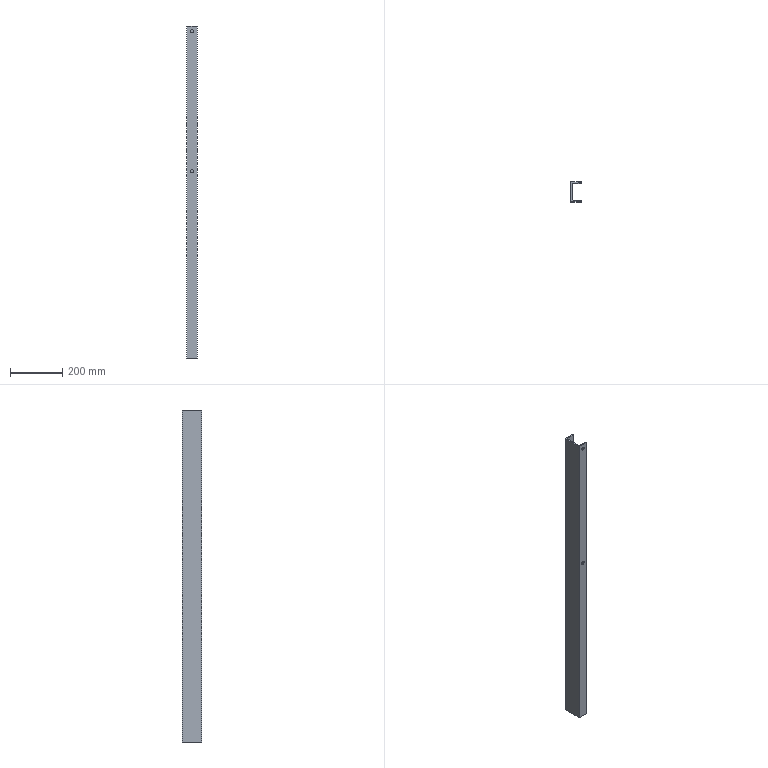Part | STEP file | BCC3 H13_6 | 1 solid | 14 faces | box 40 x 75 x 1270 mm | volume 877986 mm3 | plane 10 | cylinder 4 | commonest cylinder face diameters 12 x4
STEP:
#1=CARTESIAN_POINT('',(0.,0.,0.));
#2=DIRECTION('',(0.,0.,1.));
#3=DIRECTION('',(1.,0.,0.));
#4=AXIS2_PLACEMENT_3D('',#1,#2,#3);
#5=CARTESIAN_POINT('',(14.,-32.225,615.));
#6=VERTEX_POINT('',#5);
#7=CARTESIAN_POINT('',(14.,-37.5,615.));
#8=VERTEX_POINT('',#7);
#9=CARTESIAN_POINT('',(14.,-27.5,615.));
#10=DIRECTION('',(0.,-1.,0.));
#11=VECTOR('',#10,1.);
#12=LINE('',#9,#11);
#13=CARTESIAN_POINT('',(20.,-27.5,615.));
#14=DIRECTION('',(0.,-1.,0.));
#15=DIRECTION('',(-1.,0.,0.));
#16=AXIS2_PLACEMENT_3D('',#13,#14,#15);
#17=CYLINDRICAL_SURFACE('',#16,6.);
#18=CARTESIAN_POINT('',(6.283,0.));
#19=DIRECTION('',(0.,1.));
#20=VECTOR('',#19,1.);
#21=LINE('',#18,#20);
#22=(GEOMETRIC_REPRESENTATION_CONTEXT(2)PARAMETRIC_REPRESENTATION_CONTEXT()REPRESENTATION_CONTEXT('',''));
#23=DEFINITIONAL_REPRESENTATION('',(#21),#22);
#24=PCURVE('',#17,#23);
#25=CARTESIAN_POINT('',(20.,-27.5,615.));
#26=DIRECTION('',(0.,-1.,0.));
#27=DIRECTION('',(-1.,0.,0.));
#28=AXIS2_PLACEMENT_3D('',#25,#26,#27);
#29=CYLINDRICAL_SURFACE('',#28,6.);
#30=CARTESIAN_POINT('',(0.,0.));
#31=DIRECTION('',(0.,1.));
#32=VECTOR('',#31,1.);
#33=LINE('',#30,#32);
#34=(GEOMETRIC_REPRESENTATION_CONTEXT(2)PARAMETRIC_REPRESENTATION_CONTEXT()REPRESENTATION_CONTEXT('',''));
#35=DEFINITIONAL_REPRESENTATION('',(#33),#34);
#36=PCURVE('',#29,#35);
#37=SURFACE_CURVE('',#12,(#24,#36),.PCURVE_S1.);
#38=EDGE_CURVE('',#6,#8,#37,.T.);
#39=ORIENTED_EDGE('',*,*,#38,.T.);
#40=CARTESIAN_POINT('',(26.,-37.5,615.));
#41=VERTEX_POINT('',#40);
#42=CARTESIAN_POINT('',(20.,-37.5,615.));
#43=DIRECTION('',(0.,1.,0.));
#44=DIRECTION('',(1.,0.,0.));
#45=AXIS2_PLACEMENT_3D('',#42,#43,#44);
#46=CIRCLE('',#45,6.);
#47=CARTESIAN_POINT('',(9.425,10.));
#48=DIRECTION('',(-1.,0.));
#49=VECTOR('',#48,1.);
#50=LINE('',#47,#49);
#51=(GEOMETRIC_REPRESENTATION_CONTEXT(2)PARAMETRIC_REPRESENTATION_CONTEXT()REPRESENTATION_CONTEXT('',''));
#52=DEFINITIONAL_REPRESENTATION('',(#50),#51);
#53=PCURVE('',#17,#52);
#54=CARTESIAN_POINT('',(0.,-37.5,635.));
#55=DIRECTION('',(0.,1.,0.));
#56=DIRECTION('',(0.,0.,1.));
#57=AXIS2_PLACEMENT_3D('',#54,#55,#56);
#58=PLANE('',#57);
#59=CARTESIAN_POINT('',(-20.,20.));
#60=DIRECTION('',(0.,1.));
#61=AXIS2_PLACEMENT_2D('',#59,#60);
#62=CIRCLE('',#61,6.);
#63=(GEOMETRIC_REPRESENTATION_CONTEXT(2)PARAMETRIC_REPRESENTATION_CONTEXT()REPRESENTATION_CONTEXT('',''));
#64=DEFINITIONAL_REPRESENTATION('',(#62),#63);
#65=PCURVE('',#58,#64);
#66=SURFACE_CURVE('',#46,(#53,#65),.PCURVE_S1.);
#67=EDGE_CURVE('',#8,#41,#66,.T.);
#68=ORIENTED_EDGE('',*,*,#67,.T.);
#69=CARTESIAN_POINT('',(26.,-33.275,615.));
#70=VERTEX_POINT('',#69);
#71=CARTESIAN_POINT('',(26.,-27.5,615.));
#72=DIRECTION('',(0.,-1.,0.));
#73=VECTOR('',#72,1.);
#74=LINE('',#71,#73);
#75=CARTESIAN_POINT('',(3.142,0.));
#76=DIRECTION('',(0.,1.));
#77=VECTOR('',#76,1.);
#78=LINE('',#75,#77);
#79=(GEOMETRIC_REPRESENTATION_CONTEXT(2)PARAMETRIC_REPRESENTATION_CONTEXT()REPRESENTATION_CONTEXT('',''));
#80=DEFINITIONAL_REPRESENTATION('',(#78),#79);
#81=PCURVE('',#17,#80);
#82=CARTESIAN_POINT('',(3.142,0.));
#83=DIRECTION('',(0.,1.));
#84=VECTOR('',#83,1.);
#85=LINE('',#82,#84);
#86=(GEOMETRIC_REPRESENTATION_CONTEXT(2)PARAMETRIC_REPRESENTATION_CONTEXT()REPRESENTATION_CONTEXT('',''));
#87=DEFINITIONAL_REPRESENTATION('',(#85),#86);
#88=PCURVE('',#29,#87);
#89=SURFACE_CURVE('',#74,(#81,#88),.PCURVE_S1.);
#90=EDGE_CURVE('',#70,#41,#89,.T.);
#91=ORIENTED_EDGE('',*,*,#90,.F.);
#92=CARTESIAN_POINT('',(14.,-32.225,615.));
#93=CARTESIAN_POINT('',(14.,-32.225,627.));
#94=CARTESIAN_POINT('',(26.,-33.275,627.));
#95=CARTESIAN_POINT('',(26.,-33.275,615.));
#96=(BOUNDED_CURVE()B_SPLINE_CURVE(3,(#92,#93,#94,#95),.UNSPECIFIED.,.F.,.F.)B_SPLINE_CURVE_WITH_KNOTS((4,4),(3.142,6.283),.PIECEWISE_BEZIER_KNOTS.)CURVE()GEOMETRIC_REPRESENTATION_ITEM()RATIONAL_B_SPLINE_CURVE((1.,0.3333,0.3333,1.))REPRESENTATION_ITEM(''));
#97=CARTESIAN_POINT('',(6.283,4.725));
#98=CARTESIAN_POINT('',(6.253,4.725));
#99=CARTESIAN_POINT('',(6.19,4.727));
#100=CARTESIAN_POINT('',(6.085,4.735));
#101=CARTESIAN_POINT('',(5.972,4.749));
#102=CARTESIAN_POINT('',(5.848,4.773));
#103=CARTESIAN_POINT('',(5.713,4.807));
#104=CARTESIAN_POINT('',(5.567,4.853));
#105=CARTESIAN_POINT('',(5.412,4.911));
#106=CARTESIAN_POINT('',(5.246,4.982));
#107=CARTESIAN_POINT('',(5.073,5.064));
#108=CARTESIAN_POINT('',(4.894,5.155));
#109=CARTESIAN_POINT('',(4.712,5.25));
#110=CARTESIAN_POINT('',(4.531,5.346));
#111=CARTESIAN_POINT('',(4.352,5.436));
#112=CARTESIAN_POINT('',(4.179,5.519));
#113=CARTESIAN_POINT('',(4.013,5.59));
#114=CARTESIAN_POINT('',(3.857,5.648));
#115=CARTESIAN_POINT('',(3.712,5.694));
#116=CARTESIAN_POINT('',(3.577,5.727));
#117=CARTESIAN_POINT('',(3.453,5.751));
#118=CARTESIAN_POINT('',(3.339,5.766));
#119=CARTESIAN_POINT('',(3.235,5.774));
#120=CARTESIAN_POINT('',(3.172,5.775));
#121=CARTESIAN_POINT('',(3.142,5.775));
#122=B_SPLINE_CURVE_WITH_KNOTS('',3,(#97,#98,#99,#100,#101,#102,#103,#104,#105,#106,#107,#108,#109,#110,#111,#112,#113,#114,#115,#116,#117,#118,#119,#120,#121),.UNSPECIFIED.,.F.,.F.,(4,1,1,1,1,1,1,1,1,1,1,1,1,1,1,1,1,1,1,1,1,1,4),(3.142,3.284,3.427,3.57,3.713,3.856,3.998,4.141,4.284,4.427,4.57,4.712,4.855,4.998,5.141,5.284,5.426,5.569,5.712,5.855,5.998,6.14,6.283),.QUASI_UNIFORM_KNOTS.);
#123=(GEOMETRIC_REPRESENTATION_CONTEXT(2)PARAMETRIC_REPRESENTATION_CONTEXT()REPRESENTATION_CONTEXT('',''));
#124=DEFINITIONAL_REPRESENTATION('',(#122),#123);
#125=PCURVE('',#17,#124);
#126=CARTESIAN_POINT('',(40.,-34.5,635.));
#127=DIRECTION('',(-0.08716,-0.9962,0.));
#128=DIRECTION('',(0.9962,-0.08716,0.));
#129=AXIS2_PLACEMENT_3D('',#126,#127,#128);
#130=PLANE('',#129);
#131=CARTESIAN_POINT('',(-26.099,-20.));
#132=CARTESIAN_POINT('',(-26.099,-8.));
#133=CARTESIAN_POINT('',(-14.053,-8.));
#134=CARTESIAN_POINT('',(-14.053,-20.));
#135=(BOUNDED_CURVE()B_SPLINE_CURVE(3,(#131,#132,#133,#134),.UNSPECIFIED.,.F.,.F.)B_SPLINE_CURVE_WITH_KNOTS((4,4),(3.142,6.283),.PIECEWISE_BEZIER_KNOTS.)CURVE()GEOMETRIC_REPRESENTATION_ITEM()RATIONAL_B_SPLINE_CURVE((1.,0.3333,0.3333,1.))REPRESENTATION_ITEM(''));
#136=(GEOMETRIC_REPRESENTATION_CONTEXT(2)PARAMETRIC_REPRESENTATION_CONTEXT()REPRESENTATION_CONTEXT('',''));
#137=DEFINITIONAL_REPRESENTATION('',(#135),#136);
#138=PCURVE('',#130,#137);
#139=SURFACE_CURVE('',#96,(#125,#138),.PCURVE_S1.);
#140=EDGE_CURVE('',#6,#70,#139,.T.);
#141=ORIENTED_EDGE('',*,*,#140,.F.);
#142=EDGE_LOOP('',(#39,#68,#91,#141));
#143=FACE_BOUND('',#142,.F.);
#144=ADVANCED_FACE('',(#143),#17,.F.);
#145=CARTESIAN_POINT('',(14.,-32.225,80.));
#146=VERTEX_POINT('',#145);
#147=CARTESIAN_POINT('',(14.,-37.5,80.));
#148=VERTEX_POINT('',#147);
#149=CARTESIAN_POINT('',(14.,-27.5,80.));
#150=DIRECTION('',(0.,-1.,0.));
#151=VECTOR('',#150,1.);
#152=LINE('',#149,#151);
#153=CARTESIAN_POINT('',(20.,-27.5,80.));
#154=DIRECTION('',(0.,-1.,0.));
#155=DIRECTION('',(-1.,0.,0.));
#156=AXIS2_PLACEMENT_3D('',#153,#154,#155);
#157=CYLINDRICAL_SURFACE('',#156,6.);
#158=CARTESIAN_POINT('',(6.283,0.));
#159=DIRECTION('',(0.,1.));
#160=VECTOR('',#159,1.);
#161=LINE('',#158,#160);
#162=(GEOMETRIC_REPRESENTATION_CONTEXT(2)PARAMETRIC_REPRESENTATION_CONTEXT()REPRESENTATION_CONTEXT('',''));
#163=DEFINITIONAL_REPRESENTATION('',(#161),#162);
#164=PCURVE('',#157,#163);
#165=CARTESIAN_POINT('',(20.,-27.5,80.));
#166=DIRECTION('',(0.,-1.,0.));
#167=DIRECTION('',(-1.,0.,0.));
#168=AXIS2_PLACEMENT_3D('',#165,#166,#167);
#169=CYLINDRICAL_SURFACE('',#168,6.);
#170=CARTESIAN_POINT('',(0.,0.));
#171=DIRECTION('',(0.,1.));
#172=VECTOR('',#171,1.);
#173=LINE('',#170,#172);
#174=(GEOMETRIC_REPRESENTATION_CONTEXT(2)PARAMETRIC_REPRESENTATION_CONTEXT()REPRESENTATION_CONTEXT('',''));
#175=DEFINITIONAL_REPRESENTATION('',(#173),#174);
#176=PCURVE('',#169,#175);
#177=SURFACE_CURVE('',#152,(#164,#176),.PCURVE_S1.);
#178=EDGE_CURVE('',#146,#148,#177,.T.);
#179=ORIENTED_EDGE('',*,*,#178,.T.);
#180=CARTESIAN_POINT('',(26.,-37.5,80.));
#181=VERTEX_POINT('',#180);
#182=CARTESIAN_POINT('',(20.,-37.5,80.));
#183=DIRECTION('',(0.,1.,0.));
#184=DIRECTION('',(1.,0.,0.));
#185=AXIS2_PLACEMENT_3D('',#182,#183,#184);
#186=CIRCLE('',#185,6.);
#187=CARTESIAN_POINT('',(9.425,10.));
#188=DIRECTION('',(-1.,0.));
#189=VECTOR('',#188,1.);
#190=LINE('',#187,#189);
#191=(GEOMETRIC_REPRESENTATION_CONTEXT(2)PARAMETRIC_REPRESENTATION_CONTEXT()REPRESENTATION_CONTEXT('',''));
#192=DEFINITIONAL_REPRESENTATION('',(#190),#191);
#193=PCURVE('',#157,#192);
#194=CARTESIAN_POINT('',(-555.,20.));
#195=DIRECTION('',(0.,1.));
#196=AXIS2_PLACEMENT_2D('',#194,#195);
#197=CIRCLE('',#196,6.);
#198=(GEOMETRIC_REPRESENTATION_CONTEXT(2)PARAMETRIC_REPRESENTATION_CONTEXT()REPRESENTATION_CONTEXT('',''));
#199=DEFINITIONAL_REPRESENTATION('',(#197),#198);
#200=PCURVE('',#58,#199);
#201=SURFACE_CURVE('',#186,(#193,#200),.PCURVE_S1.);
#202=EDGE_CURVE('',#148,#181,#201,.T.);
#203=ORIENTED_EDGE('',*,*,#202,.T.);
#204=CARTESIAN_POINT('',(26.,-33.275,80.));
#205=VERTEX_POINT('',#204);
#206=CARTESIAN_POINT('',(26.,-27.5,80.));
#207=DIRECTION('',(0.,-1.,0.));
#208=VECTOR('',#207,1.);
#209=LINE('',#206,#208);
#210=CARTESIAN_POINT('',(3.142,0.));
#211=DIRECTION('',(0.,1.));
#212=VECTOR('',#211,1.);
#213=LINE('',#210,#212);
#214=(GEOMETRIC_REPRESENTATION_CONTEXT(2)PARAMETRIC_REPRESENTATION_CONTEXT()REPRESENTATION_CONTEXT('',''));
#215=DEFINITIONAL_REPRESENTATION('',(#213),#214);
#216=PCURVE('',#157,#215);
#217=CARTESIAN_POINT('',(3.142,0.));
#218=DIRECTION('',(0.,1.));
#219=VECTOR('',#218,1.);
#220=LINE('',#217,#219);
#221=(GEOMETRIC_REPRESENTATION_CONTEXT(2)PARAMETRIC_REPRESENTATION_CONTEXT()REPRESENTATION_CONTEXT('',''));
#222=DEFINITIONAL_REPRESENTATION('',(#220),#221);
#223=PCURVE('',#169,#222);
#224=SURFACE_CURVE('',#209,(#216,#223),.PCURVE_S1.);
#225=EDGE_CURVE('',#205,#181,#224,.T.);
#226=ORIENTED_EDGE('',*,*,#225,.F.);
#227=CARTESIAN_POINT('',(14.,-32.225,80.));
#228=CARTESIAN_POINT('',(14.,-32.225,92.));
#229=CARTESIAN_POINT('',(26.,-33.275,92.));
#230=CARTESIAN_POINT('',(26.,-33.275,80.));
#231=(BOUNDED_CURVE()B_SPLINE_CURVE(3,(#227,#228,#229,#230),.UNSPECIFIED.,.F.,.F.)B_SPLINE_CURVE_WITH_KNOTS((4,4),(3.142,6.283),.PIECEWISE_BEZIER_KNOTS.)CURVE()GEOMETRIC_REPRESENTATION_ITEM()RATIONAL_B_SPLINE_CURVE((1.,0.3333,0.3333,1.))REPRESENTATION_ITEM(''));
#232=CARTESIAN_POINT('',(6.283,4.725));
#233=CARTESIAN_POINT('',(6.253,4.725));
#234=CARTESIAN_POINT('',(6.19,4.727));
#235=CARTESIAN_POINT('',(6.085,4.735));
#236=CARTESIAN_POINT('',(5.972,4.749));
#237=CARTESIAN_POINT('',(5.848,4.773));
#238=CARTESIAN_POINT('',(5.713,4.807));
#239=CARTESIAN_POINT('',(5.567,4.853));
#240=CARTESIAN_POINT('',(5.412,4.911));
#241=CARTESIAN_POINT('',(5.246,4.982));
#242=CARTESIAN_POINT('',(5.073,5.064));
#243=CARTESIAN_POINT('',(4.894,5.155));
#244=CARTESIAN_POINT('',(4.712,5.25));
#245=CARTESIAN_POINT('',(4.531,5.346));
#246=CARTESIAN_POINT('',(4.352,5.436));
#247=CARTESIAN_POINT('',(4.179,5.519));
#248=CARTESIAN_POINT('',(4.013,5.59));
#249=CARTESIAN_POINT('',(3.857,5.648));
#250=CARTESIAN_POINT('',(3.712,5.694));
#251=CARTESIAN_POINT('',(3.577,5.727));
#252=CARTESIAN_POINT('',(3.453,5.751));
#253=CARTESIAN_POINT('',(3.339,5.766));
#254=CARTESIAN_POINT('',(3.235,5.774));
#255=CARTESIAN_POINT('',(3.172,5.775));
#256=CARTESIAN_POINT('',(3.142,5.775));
#257=B_SPLINE_CURVE_WITH_KNOTS('',3,(#232,#233,#234,#235,#236,#237,#238,#239,#240,#241,#242,#243,#244,#245,#246,#247,#248,#249,#250,#251,#252,#253,#254,#255,#256),.UNSPECIFIED.,.F.,.F.,(4,1,1,1,1,1,1,1,1,1,1,1,1,1,1,1,1,1,1,1,1,1,4),(3.142,3.284,3.427,3.57,3.713,3.856,3.998,4.141,4.284,4.427,4.57,4.712,4.855,4.998,5.141,5.284,5.426,5.569,5.712,5.855,5.998,6.14,6.283),.QUASI_UNIFORM_KNOTS.);
#258=(GEOMETRIC_REPRESENTATION_CONTEXT(2)PARAMETRIC_REPRESENTATION_CONTEXT()REPRESENTATION_CONTEXT('',''));
#259=DEFINITIONAL_REPRESENTATION('',(#257),#258);
#260=PCURVE('',#157,#259);
#261=CARTESIAN_POINT('',(-26.099,-555.));
#262=CARTESIAN_POINT('',(-26.099,-543.));
#263=CARTESIAN_POINT('',(-14.053,-543.));
#264=CARTESIAN_POINT('',(-14.053,-555.));
#265=(BOUNDED_CURVE()B_SPLINE_CURVE(3,(#261,#262,#263,#264),.UNSPECIFIED.,.F.,.F.)B_SPLINE_CURVE_WITH_KNOTS((4,4),(3.142,6.283),.PIECEWISE_BEZIER_KNOTS.)CURVE()GEOMETRIC_REPRESENTATION_ITEM()RATIONAL_B_SPLINE_CURVE((1.,0.3333,0.3333,1.))REPRESENTATION_ITEM(''));
#266=(GEOMETRIC_REPRESENTATION_CONTEXT(2)PARAMETRIC_REPRESENTATION_CONTEXT()REPRESENTATION_CONTEXT('',''));
#267=DEFINITIONAL_REPRESENTATION('',(#265),#266);
#268=PCURVE('',#130,#267);
#269=SURFACE_CURVE('',#231,(#260,#268),.PCURVE_S1.);
#270=EDGE_CURVE('',#146,#205,#269,.T.);
#271=ORIENTED_EDGE('',*,*,#270,.F.);
#272=EDGE_LOOP('',(#179,#203,#226,#271));
#273=FACE_BOUND('',#272,.F.);
#274=ADVANCED_FACE('',(#273),#157,.F.);
#275=ORIENTED_EDGE('',*,*,#202,.T.);
#276=CARTESIAN_POINT('',(20.,-37.5,80.));
#277=DIRECTION('',(0.,1.,0.));
#278=DIRECTION('',(1.,0.,0.));
#279=AXIS2_PLACEMENT_3D('',#276,#277,#278);
#280=CIRCLE('',#279,6.);
#281=CARTESIAN_POINT('',(-555.,20.));
#282=DIRECTION('',(0.,1.));
#283=AXIS2_PLACEMENT_2D('',#281,#282);
#284=CIRCLE('',#283,6.);
#285=(GEOMETRIC_REPRESENTATION_CONTEXT(2)PARAMETRIC_REPRESENTATION_CONTEXT()REPRESENTATION_CONTEXT('',''));
#286=DEFINITIONAL_REPRESENTATION('',(#284),#285);
#287=PCURVE('',#58,#286);
#288=CARTESIAN_POINT('',(3.142,10.));
#289=DIRECTION('',(-1.,0.));
#290=VECTOR('',#289,1.);
#291=LINE('',#288,#290);
#292=(GEOMETRIC_REPRESENTATION_CONTEXT(2)PARAMETRIC_REPRESENTATION_CONTEXT()REPRESENTATION_CONTEXT('',''));
#293=DEFINITIONAL_REPRESENTATION('',(#291),#292);
#294=PCURVE('',#169,#293);
#295=SURFACE_CURVE('',#280,(#287,#294),.PCURVE_S1.);
#296=EDGE_CURVE('',#181,#148,#295,.T.);
#297=ORIENTED_EDGE('',*,*,#296,.T.);
#298=EDGE_LOOP('',(#275,#297));
#299=FACE_BOUND('',#298,.T.);
#300=CARTESIAN_POINT('',(0.,-37.5,-635.));
#301=VERTEX_POINT('',#300);
#302=CARTESIAN_POINT('',(40.,-37.5,-635.));
#303=VERTEX_POINT('',#302);
#304=CARTESIAN_POINT('',(0.,-37.5,-635.));
#305=DIRECTION('',(1.,0.,0.));
#306=VECTOR('',#305,1.);
#307=LINE('',#304,#306);
#308=CARTESIAN_POINT('',(-1270.,0.));
#309=DIRECTION('',(0.,1.));
#310=VECTOR('',#309,1.);
#311=LINE('',#308,#310);
#312=(GEOMETRIC_REPRESENTATION_CONTEXT(2)PARAMETRIC_REPRESENTATION_CONTEXT()REPRESENTATION_CONTEXT('',''));
#313=DEFINITIONAL_REPRESENTATION('',(#311),#312);
#314=PCURVE('',#58,#313);
#315=CARTESIAN_POINT('',(0.,0.,-635.));
#316=DIRECTION('',(0.,0.,1.));
#317=DIRECTION('',(1.,0.,0.));
#318=AXIS2_PLACEMENT_3D('',#315,#316,#317);
#319=PLANE('',#318);
#320=CARTESIAN_POINT('',(0.,-37.5));
#321=DIRECTION('',(1.,0.));
#322=VECTOR('',#321,1.);
#323=LINE('',#320,#322);
#324=(GEOMETRIC_REPRESENTATION_CONTEXT(2)PARAMETRIC_REPRESENTATION_CONTEXT()REPRESENTATION_CONTEXT('',''));
#325=DEFINITIONAL_REPRESENTATION('',(#323),#324);
#326=PCURVE('',#319,#325);
#327=SURFACE_CURVE('',#307,(#314,#326),.PCURVE_S1.);
#328=EDGE_CURVE('',#301,#303,#327,.T.);
#329=ORIENTED_EDGE('',*,*,#328,.T.);
#330=CARTESIAN_POINT('',(40.,-37.5,635.));
#331=VERTEX_POINT('',#330);
#332=CARTESIAN_POINT('',(40.,-37.5,635.));
#333=DIRECTION('',(0.,0.,-1.));
#334=VECTOR('',#333,1.);
#335=LINE('',#332,#334);
#336=CARTESIAN_POINT('',(0.,40.));
#337=DIRECTION('',(-1.,0.));
#338=VECTOR('',#337,1.);
#339=LINE('',#336,#338);
#340=(GEOMETRIC_REPRESENTATION_CONTEXT(2)PARAMETRIC_REPRESENTATION_CONTEXT()REPRESENTATION_CONTEXT('',''));
#341=DEFINITIONAL_REPRESENTATION('',(#339),#340);
#342=PCURVE('',#58,#341);
#343=CARTESIAN_POINT('',(40.,-37.5,635.));
#344=DIRECTION('',(-1.,0.,0.));
#345=DIRECTION('',(0.,0.,1.));
#346=AXIS2_PLACEMENT_3D('',#343,#344,#345);
#347=PLANE('',#346);
#348=CARTESIAN_POINT('',(0.,0.));
#349=DIRECTION('',(-1.,0.));
#350=VECTOR('',#349,1.);
#351=LINE('',#348,#350);
#352=(GEOMETRIC_REPRESENTATION_CONTEXT(2)PARAMETRIC_REPRESENTATION_CONTEXT()REPRESENTATION_CONTEXT('',''));
#353=DEFINITIONAL_REPRESENTATION('',(#351),#352);
#354=PCURVE('',#347,#353);
#355=SURFACE_CURVE('',#335,(#342,#354),.PCURVE_S1.);
#356=EDGE_CURVE('',#331,#303,#355,.T.);
#357=ORIENTED_EDGE('',*,*,#356,.F.);
#358=CARTESIAN_POINT('',(0.,-37.5,635.));
#359=VERTEX_POINT('',#358);
#360=CARTESIAN_POINT('',(0.,-37.5,635.));
#361=DIRECTION('',(1.,0.,0.));
#362=VECTOR('',#361,1.);
#363=LINE('',#360,#362);
#364=CARTESIAN_POINT('',(0.,0.));
#365=DIRECTION('',(0.,1.));
#366=VECTOR('',#365,1.);
#367=LINE('',#364,#366);
#368=(GEOMETRIC_REPRESENTATION_CONTEXT(2)PARAMETRIC_REPRESENTATION_CONTEXT()REPRESENTATION_CONTEXT('',''));
#369=DEFINITIONAL_REPRESENTATION('',(#367),#368);
#370=PCURVE('',#58,#369);
#371=CARTESIAN_POINT('',(0.,0.,635.));
#372=DIRECTION('',(0.,0.,1.));
#373=DIRECTION('',(1.,0.,0.));
#374=AXIS2_PLACEMENT_3D('',#371,#372,#373);
#375=PLANE('',#374);
#376=CARTESIAN_POINT('',(0.,-37.5));
#377=DIRECTION('',(1.,0.));
#378=VECTOR('',#377,1.);
#379=LINE('',#376,#378);
#380=(GEOMETRIC_REPRESENTATION_CONTEXT(2)PARAMETRIC_REPRESENTATION_CONTEXT()REPRESENTATION_CONTEXT('',''));
#381=DEFINITIONAL_REPRESENTATION('',(#379),#380);
#382=PCURVE('',#375,#381);
#383=SURFACE_CURVE('',#363,(#370,#382),.PCURVE_S1.);
#384=EDGE_CURVE('',#359,#331,#383,.T.);
#385=ORIENTED_EDGE('',*,*,#384,.F.);
#386=CARTESIAN_POINT('',(0.,-37.5,635.));
#387=DIRECTION('',(0.,0.,-1.));
#388=VECTOR('',#387,1.);
#389=LINE('',#386,#388);
#390=CARTESIAN_POINT('',(0.,0.));
#391=DIRECTION('',(-1.,0.));
#392=VECTOR('',#391,1.);
#393=LINE('',#390,#392);
#394=(GEOMETRIC_REPRESENTATION_CONTEXT(2)PARAMETRIC_REPRESENTATION_CONTEXT()REPRESENTATION_CONTEXT('',''));
#395=DEFINITIONAL_REPRESENTATION('',(#393),#394);
#396=PCURVE('',#58,#395);
#397=CARTESIAN_POINT('',(0.,37.5,635.));
#398=DIRECTION('',(1.,0.,0.));
#399=DIRECTION('',(0.,0.,-1.));
#400=AXIS2_PLACEMENT_3D('',#397,#398,#399);
#401=PLANE('',#400);
#402=CARTESIAN_POINT('',(0.,-75.));
#403=DIRECTION('',(1.,0.));
#404=VECTOR('',#403,1.);
#405=LINE('',#402,#404);
#406=(GEOMETRIC_REPRESENTATION_CONTEXT(2)PARAMETRIC_REPRESENTATION_CONTEXT()REPRESENTATION_CONTEXT('',''));
#407=DEFINITIONAL_REPRESENTATION('',(#405),#406);
#408=PCURVE('',#401,#407);
#409=SURFACE_CURVE('',#389,(#396,#408),.PCURVE_S1.);
#410=EDGE_CURVE('',#359,#301,#409,.T.);
#411=ORIENTED_EDGE('',*,*,#410,.T.);
#412=EDGE_LOOP('',(#329,#357,#385,#411));
#413=FACE_BOUND('',#412,.T.);
#414=ORIENTED_EDGE('',*,*,#67,.T.);
#415=CARTESIAN_POINT('',(20.,-37.5,615.));
#416=DIRECTION('',(0.,1.,0.));
#417=DIRECTION('',(1.,0.,0.));
#418=AXIS2_PLACEMENT_3D('',#415,#416,#417);
#419=CIRCLE('',#418,6.);
#420=CARTESIAN_POINT('',(-20.,20.));
#421=DIRECTION('',(0.,1.));
#422=AXIS2_PLACEMENT_2D('',#420,#421);
#423=CIRCLE('',#422,6.);
#424=(GEOMETRIC_REPRESENTATION_CONTEXT(2)PARAMETRIC_REPRESENTATION_CONTEXT()REPRESENTATION_CONTEXT('',''));
#425=DEFINITIONAL_REPRESENTATION('',(#423),#424);
#426=PCURVE('',#58,#425);
#427=CARTESIAN_POINT('',(3.142,10.));
#428=DIRECTION('',(-1.,0.));
#429=VECTOR('',#428,1.);
#430=LINE('',#427,#429);
#431=(GEOMETRIC_REPRESENTATION_CONTEXT(2)PARAMETRIC_REPRESENTATION_CONTEXT()REPRESENTATION_CONTEXT('',''));
#432=DEFINITIONAL_REPRESENTATION('',(#430),#431);
#433=PCURVE('',#29,#432);
#434=SURFACE_CURVE('',#419,(#426,#433),.PCURVE_S1.);
#435=EDGE_CURVE('',#41,#8,#434,.T.);
#436=ORIENTED_EDGE('',*,*,#435,.T.);
#437=EDGE_LOOP('',(#414,#436));
#438=FACE_BOUND('',#437,.T.);
#439=ADVANCED_FACE('',(#299,#413,#438),#58,.F.);
#440=ORIENTED_EDGE('',*,*,#270,.F.);
#441=CARTESIAN_POINT('',(26.,-33.275,80.));
#442=CARTESIAN_POINT('',(26.,-33.275,68.));
#443=CARTESIAN_POINT('',(14.,-32.225,68.));
#444=CARTESIAN_POINT('',(14.,-32.225,80.));
#445=(BOUNDED_CURVE()B_SPLINE_CURVE(3,(#441,#442,#443,#444),.UNSPECIFIED.,.F.,.F.)B_SPLINE_CURVE_WITH_KNOTS((4,4),(0.,3.142),.PIECEWISE_BEZIER_KNOTS.)CURVE()GEOMETRIC_REPRESENTATION_ITEM()RATIONAL_B_SPLINE_CURVE((1.,0.3333,0.3333,1.))REPRESENTATION_ITEM(''));
#446=CARTESIAN_POINT('',(-14.053,-555.));
#447=CARTESIAN_POINT('',(-14.053,-567.));
#448=CARTESIAN_POINT('',(-26.099,-567.));
#449=CARTESIAN_POINT('',(-26.099,-555.));
#450=(BOUNDED_CURVE()B_SPLINE_CURVE(3,(#446,#447,#448,#449),.UNSPECIFIED.,.F.,.F.)B_SPLINE_CURVE_WITH_KNOTS((4,4),(0.,3.142),.PIECEWISE_BEZIER_KNOTS.)CURVE()GEOMETRIC_REPRESENTATION_ITEM()RATIONAL_B_SPLINE_CURVE((1.,0.3333,0.3333,1.))REPRESENTATION_ITEM(''));
#451=(GEOMETRIC_REPRESENTATION_CONTEXT(2)PARAMETRIC_REPRESENTATION_CONTEXT()REPRESENTATION_CONTEXT('',''));
#452=DEFINITIONAL_REPRESENTATION('',(#450),#451);
#453=PCURVE('',#130,#452);
#454=CARTESIAN_POINT('',(3.142,5.775));
#455=CARTESIAN_POINT('',(3.111,5.775));
#456=CARTESIAN_POINT('',(3.048,5.774));
#457=CARTESIAN_POINT('',(2.944,5.766));
#458=CARTESIAN_POINT('',(2.83,5.751));
#459=CARTESIAN_POINT('',(2.706,5.727));
#460=CARTESIAN_POINT('',(2.571,5.694));
#461=CARTESIAN_POINT('',(2.426,5.648));
#462=CARTESIAN_POINT('',(2.27,5.59));
#463=CARTESIAN_POINT('',(2.105,5.519));
#464=CARTESIAN_POINT('',(1.931,5.436));
#465=CARTESIAN_POINT('',(1.753,5.346));
#466=CARTESIAN_POINT('',(1.571,5.25));
#467=CARTESIAN_POINT('',(1.389,5.155));
#468=CARTESIAN_POINT('',(1.21,5.064));
#469=CARTESIAN_POINT('',(1.037,4.982));
#470=CARTESIAN_POINT('',(0.8717,4.911));
#471=CARTESIAN_POINT('',(0.7158,4.853));
#472=CARTESIAN_POINT('',(0.5703,4.807));
#473=CARTESIAN_POINT('',(0.4356,4.773));
#474=CARTESIAN_POINT('',(0.3115,4.749));
#475=CARTESIAN_POINT('',(0.1977,4.735));
#476=CARTESIAN_POINT('',(0.09367,4.727));
#477=CARTESIAN_POINT('',(0.0303,4.725));
#478=CARTESIAN_POINT('',(0.,4.725));
#479=B_SPLINE_CURVE_WITH_KNOTS('',3,(#454,#455,#456,#457,#458,#459,#460,#461,#462,#463,#464,#465,#466,#467,#468,#469,#470,#471,#472,#473,#474,#475,#476,#477,#478),.UNSPECIFIED.,.F.,.F.,(4,1,1,1,1,1,1,1,1,1,1,1,1,1,1,1,1,1,1,1,1,1,4),(0.,0.1428,0.2856,0.4284,0.5712,0.714,0.8568,0.9996,1.142,1.285,1.428,1.571,1.714,1.856,1.999,2.142,2.285,2.428,2.57,2.713,2.856,2.999,3.142),.QUASI_UNIFORM_KNOTS.);
#480=(GEOMETRIC_REPRESENTATION_CONTEXT(2)PARAMETRIC_REPRESENTATION_CONTEXT()REPRESENTATION_CONTEXT('',''));
#481=DEFINITIONAL_REPRESENTATION('',(#479),#480);
#482=PCURVE('',#169,#481);
#483=SURFACE_CURVE('',#445,(#453,#482),.PCURVE_S1.);
#484=EDGE_CURVE('',#205,#146,#483,.T.);
#485=ORIENTED_EDGE('',*,*,#484,.F.);
#486=EDGE_LOOP('',(#440,#485));
#487=FACE_BOUND('',#486,.T.);
#488=CARTESIAN_POINT('',(40.,-34.5,-635.));
#489=VERTEX_POINT('',#488);
#490=CARTESIAN_POINT('',(5.,-31.438,-635.));
#491=VERTEX_POINT('',#490);
#492=CARTESIAN_POINT('',(40.,-34.5,-635.));
#493=DIRECTION('',(-0.9962,0.08716,0.));
#494=VECTOR('',#493,1.);
#495=LINE('',#492,#494);
#496=CARTESIAN_POINT('',(0.,-1270.));
#497=DIRECTION('',(-1.,0.));
#498=VECTOR('',#497,1.);
#499=LINE('',#496,#498);
#500=(GEOMETRIC_REPRESENTATION_CONTEXT(2)PARAMETRIC_REPRESENTATION_CONTEXT()REPRESENTATION_CONTEXT('',''));
#501=DEFINITIONAL_REPRESENTATION('',(#499),#500);
#502=PCURVE('',#130,#501);
#503=CARTESIAN_POINT('',(40.,-34.5));
#504=DIRECTION('',(-0.9962,0.08716));
#505=VECTOR('',#504,1.);
#506=LINE('',#503,#505);
#507=(GEOMETRIC_REPRESENTATION_CONTEXT(2)PARAMETRIC_REPRESENTATION_CONTEXT()REPRESENTATION_CONTEXT('',''));
#508=DEFINITIONAL_REPRESENTATION('',(#506),#507);
#509=PCURVE('',#319,#508);
#510=SURFACE_CURVE('',#495,(#502,#509),.PCURVE_S1.);
#511=EDGE_CURVE('',#489,#491,#510,.T.);
#512=ORIENTED_EDGE('',*,*,#511,.T.);
#513=CARTESIAN_POINT('',(5.,-31.438,635.));
#514=VERTEX_POINT('',#513);
#515=CARTESIAN_POINT('',(5.,-31.438,635.));
#516=DIRECTION('',(0.,0.,-1.));
#517=VECTOR('',#516,1.);
#518=LINE('',#515,#517);
#519=CARTESIAN_POINT('',(-35.134,0.));
#520=DIRECTION('',(0.,-1.));
#521=VECTOR('',#520,1.);
#522=LINE('',#519,#521);
#523=(GEOMETRIC_REPRESENTATION_CONTEXT(2)PARAMETRIC_REPRESENTATION_CONTEXT()REPRESENTATION_CONTEXT('',''));
#524=DEFINITIONAL_REPRESENTATION('',(#522),#523);
#525=PCURVE('',#130,#524);
#526=CARTESIAN_POINT('',(5.,-31.438,635.));
#527=DIRECTION('',(-1.,0.,0.));
#528=DIRECTION('',(0.,0.,1.));
#529=AXIS2_PLACEMENT_3D('',#526,#527,#528);
#530=PLANE('',#529);
#531=CARTESIAN_POINT('',(0.,0.));
#532=DIRECTION('',(-1.,0.));
#533=VECTOR('',#532,1.);
#534=LINE('',#531,#533);
#535=(GEOMETRIC_REPRESENTATION_CONTEXT(2)PARAMETRIC_REPRESENTATION_CONTEXT()REPRESENTATION_CONTEXT('',''));
#536=DEFINITIONAL_REPRESENTATION('',(#534),#535);
#537=PCURVE('',#530,#536);
#538=SURFACE_CURVE('',#518,(#525,#537),.PCURVE_S1.);
#539=EDGE_CURVE('',#514,#491,#538,.T.);
#540=ORIENTED_EDGE('',*,*,#539,.F.);
#541=CARTESIAN_POINT('',(40.,-34.5,635.));
#542=VERTEX_POINT('',#541);
#543=CARTESIAN_POINT('',(40.,-34.5,635.));
#544=DIRECTION('',(-0.9962,0.08716,0.));
#545=VECTOR('',#544,1.);
#546=LINE('',#543,#545);
#547=CARTESIAN_POINT('',(0.,0.));
#548=DIRECTION('',(-1.,0.));
#549=VECTOR('',#548,1.);
#550=LINE('',#547,#549);
#551=(GEOMETRIC_REPRESENTATION_CONTEXT(2)PARAMETRIC_REPRESENTATION_CONTEXT()REPRESENTATION_CONTEXT('',''));
#552=DEFINITIONAL_REPRESENTATION('',(#550),#551);
#553=PCURVE('',#130,#552);
#554=CARTESIAN_POINT('',(40.,-34.5));
#555=DIRECTION('',(-0.9962,0.08716));
#556=VECTOR('',#555,1.);
#557=LINE('',#554,#556);
#558=(GEOMETRIC_REPRESENTATION_CONTEXT(2)PARAMETRIC_REPRESENTATION_CONTEXT()REPRESENTATION_CONTEXT('',''));
#559=DEFINITIONAL_REPRESENTATION('',(#557),#558);
#560=PCURVE('',#375,#559);
#561=SURFACE_CURVE('',#546,(#553,#560),.PCURVE_S1.);
#562=EDGE_CURVE('',#542,#514,#561,.T.);
#563=ORIENTED_EDGE('',*,*,#562,.F.);
#564=CARTESIAN_POINT('',(40.,-34.5,635.));
#565=DIRECTION('',(0.,0.,-1.));
#566=VECTOR('',#565,1.);
#567=LINE('',#564,#566);
#568=CARTESIAN_POINT('',(0.,0.));
#569=DIRECTION('',(0.,-1.));
#570=VECTOR('',#569,1.);
#571=LINE('',#568,#570);
#572=(GEOMETRIC_REPRESENTATION_CONTEXT(2)PARAMETRIC_REPRESENTATION_CONTEXT()REPRESENTATION_CONTEXT('',''));
#573=DEFINITIONAL_REPRESENTATION('',(#571),#572);
#574=PCURVE('',#130,#573);
#575=CARTESIAN_POINT('',(0.,3.));
#576=DIRECTION('',(-1.,0.));
#577=VECTOR('',#576,1.);
#578=LINE('',#575,#577);
#579=(GEOMETRIC_REPRESENTATION_CONTEXT(2)PARAMETRIC_REPRESENTATION_CONTEXT()REPRESENTATION_CONTEXT('',''));
#580=DEFINITIONAL_REPRESENTATION('',(#578),#579);
#581=PCURVE('',#347,#580);
#582=SURFACE_CURVE('',#567,(#574,#581),.PCURVE_S1.);
#583=EDGE_CURVE('',#542,#489,#582,.T.);
#584=ORIENTED_EDGE('',*,*,#583,.T.);
#585=EDGE_LOOP('',(#512,#540,#563,#584));
#586=FACE_BOUND('',#585,.T.);
#587=ORIENTED_EDGE('',*,*,#140,.F.);
#588=CARTESIAN_POINT('',(26.,-33.275,615.));
#589=CARTESIAN_POINT('',(26.,-33.275,603.));
#590=CARTESIAN_POINT('',(14.,-32.225,603.));
#591=CARTESIAN_POINT('',(14.,-32.225,615.));
#592=(BOUNDED_CURVE()B_SPLINE_CURVE(3,(#588,#589,#590,#591),.UNSPECIFIED.,.F.,.F.)B_SPLINE_CURVE_WITH_KNOTS((4,4),(0.,3.142),.PIECEWISE_BEZIER_KNOTS.)CURVE()GEOMETRIC_REPRESENTATION_ITEM()RATIONAL_B_SPLINE_CURVE((1.,0.3333,0.3333,1.))REPRESENTATION_ITEM(''));
#593=CARTESIAN_POINT('',(-14.053,-20.));
#594=CARTESIAN_POINT('',(-14.053,-32.));
#595=CARTESIAN_POINT('',(-26.099,-32.));
#596=CARTESIAN_POINT('',(-26.099,-20.));
#597=(BOUNDED_CURVE()B_SPLINE_CURVE(3,(#593,#594,#595,#596),.UNSPECIFIED.,.F.,.F.)B_SPLINE_CURVE_WITH_KNOTS((4,4),(0.,3.142),.PIECEWISE_BEZIER_KNOTS.)CURVE()GEOMETRIC_REPRESENTATION_ITEM()RATIONAL_B_SPLINE_CURVE((1.,0.3333,0.3333,1.))REPRESENTATION_ITEM(''));
#598=(GEOMETRIC_REPRESENTATION_CONTEXT(2)PARAMETRIC_REPRESENTATION_CONTEXT()REPRESENTATION_CONTEXT('',''));
#599=DEFINITIONAL_REPRESENTATION('',(#597),#598);
#600=PCURVE('',#130,#599);
#601=CARTESIAN_POINT('',(3.142,5.775));
#602=CARTESIAN_POINT('',(3.111,5.775));
#603=CARTESIAN_POINT('',(3.048,5.774));
#604=CARTESIAN_POINT('',(2.944,5.766));
#605=CARTESIAN_POINT('',(2.83,5.751));
#606=CARTESIAN_POINT('',(2.706,5.727));
#607=CARTESIAN_POINT('',(2.571,5.694));
#608=CARTESIAN_POINT('',(2.426,5.648));
#609=CARTESIAN_POINT('',(2.27,5.59));
#610=CARTESIAN_POINT('',(2.105,5.519));
#611=CARTESIAN_POINT('',(1.931,5.436));
#612=CARTESIAN_POINT('',(1.753,5.346));
#613=CARTESIAN_POINT('',(1.571,5.25));
#614=CARTESIAN_POINT('',(1.389,5.155));
#615=CARTESIAN_POINT('',(1.21,5.064));
#616=CARTESIAN_POINT('',(1.037,4.982));
#617=CARTESIAN_POINT('',(0.8717,4.911));
#618=CARTESIAN_POINT('',(0.7158,4.853));
#619=CARTESIAN_POINT('',(0.5703,4.807));
#620=CARTESIAN_POINT('',(0.4356,4.773));
#621=CARTESIAN_POINT('',(0.3115,4.749));
#622=CARTESIAN_POINT('',(0.1977,4.735));
#623=CARTESIAN_POINT('',(0.09367,4.727));
#624=CARTESIAN_POINT('',(0.0303,4.725));
#625=CARTESIAN_POINT('',(0.,4.725));
#626=B_SPLINE_CURVE_WITH_KNOTS('',3,(#601,#602,#603,#604,#605,#606,#607,#608,#609,#610,#611,#612,#613,#614,#615,#616,#617,#618,#619,#620,#621,#622,#623,#624,#625),.UNSPECIFIED.,.F.,.F.,(4,1,1,1,1,1,1,1,1,1,1,1,1,1,1,1,1,1,1,1,1,1,4),(0.,0.1428,0.2856,0.4284,0.5712,0.714,0.8568,0.9996,1.142,1.285,1.428,1.571,1.714,1.856,1.999,2.142,2.285,2.428,2.57,2.713,2.856,2.999,3.142),.QUASI_UNIFORM_KNOTS.);
#627=(GEOMETRIC_REPRESENTATION_CONTEXT(2)PARAMETRIC_REPRESENTATION_CONTEXT()REPRESENTATION_CONTEXT('',''));
#628=DEFINITIONAL_REPRESENTATION('',(#626),#627);
#629=PCURVE('',#29,#628);
#630=SURFACE_CURVE('',#592,(#600,#629),.PCURVE_S1.);
#631=EDGE_CURVE('',#70,#6,#630,.T.);
#632=ORIENTED_EDGE('',*,*,#631,.F.);
#633=EDGE_LOOP('',(#587,#632));
#634=FACE_BOUND('',#633,.T.);
#635=ADVANCED_FACE('',(#487,#586,#634),#130,.F.);
#636=CARTESIAN_POINT('',(40.,37.5,-635.));
#637=VERTEX_POINT('',#636);
#638=CARTESIAN_POINT('',(0.,37.5,-635.));
#639=VERTEX_POINT('',#638);
#640=CARTESIAN_POINT('',(40.,37.5,-635.));
#641=DIRECTION('',(-1.,0.,0.));
#642=VECTOR('',#641,1.);
#643=LINE('',#640,#642);
#644=CARTESIAN_POINT('',(40.,37.5,635.));
#645=DIRECTION('',(0.,-1.,0.));
#646=DIRECTION('',(0.,0.,-1.));
#647=AXIS2_PLACEMENT_3D('',#644,#645,#646);
#648=PLANE('',#647);
#649=CARTESIAN_POINT('',(1270.,0.));
#650=DIRECTION('',(0.,-1.));
#651=VECTOR('',#650,1.);
#652=LINE('',#649,#651);
#653=(GEOMETRIC_REPRESENTATION_CONTEXT(2)PARAMETRIC_REPRESENTATION_CONTEXT()REPRESENTATION_CONTEXT('',''));
#654=DEFINITIONAL_REPRESENTATION('',(#652),#653);
#655=PCURVE('',#648,#654);
#656=CARTESIAN_POINT('',(40.,37.5));
#657=DIRECTION('',(-1.,0.));
#658=VECTOR('',#657,1.);
#659=LINE('',#656,#658);
#660=(GEOMETRIC_REPRESENTATION_CONTEXT(2)PARAMETRIC_REPRESENTATION_CONTEXT()REPRESENTATION_CONTEXT('',''));
#661=DEFINITIONAL_REPRESENTATION('',(#659),#660);
#662=PCURVE('',#319,#661);
#663=SURFACE_CURVE('',#643,(#655,#662),.PCURVE_S1.);
#664=EDGE_CURVE('',#637,#639,#663,.T.);
#665=ORIENTED_EDGE('',*,*,#664,.T.);
#666=CARTESIAN_POINT('',(0.,37.5,635.));
#667=VERTEX_POINT('',#666);
#668=CARTESIAN_POINT('',(0.,37.5,635.));
#669=DIRECTION('',(0.,0.,-1.));
#670=VECTOR('',#669,1.);
#671=LINE('',#668,#670);
#672=CARTESIAN_POINT('',(0.,-40.));
#673=DIRECTION('',(1.,0.));
#674=VECTOR('',#673,1.);
#675=LINE('',#672,#674);
#676=(GEOMETRIC_REPRESENTATION_CONTEXT(2)PARAMETRIC_REPRESENTATION_CONTEXT()REPRESENTATION_CONTEXT('',''));
#677=DEFINITIONAL_REPRESENTATION('',(#675),#676);
#678=PCURVE('',#648,#677);
#679=CARTESIAN_POINT('',(0.,0.));
#680=DIRECTION('',(1.,0.));
#681=VECTOR('',#680,1.);
#682=LINE('',#679,#681);
#683=(GEOMETRIC_REPRESENTATION_CONTEXT(2)PARAMETRIC_REPRESENTATION_CONTEXT()REPRESENTATION_CONTEXT('',''));
#684=DEFINITIONAL_REPRESENTATION('',(#682),#683);
#685=PCURVE('',#401,#684);
#686=SURFACE_CURVE('',#671,(#678,#685),.PCURVE_S1.);
#687=EDGE_CURVE('',#667,#639,#686,.T.);
#688=ORIENTED_EDGE('',*,*,#687,.F.);
#689=CARTESIAN_POINT('',(40.,37.5,635.));
#690=VERTEX_POINT('',#689);
#691=CARTESIAN_POINT('',(40.,37.5,635.));
#692=DIRECTION('',(-1.,0.,0.));
#693=VECTOR('',#692,1.);
#694=LINE('',#691,#693);
#695=CARTESIAN_POINT('',(0.,0.));
#696=DIRECTION('',(0.,-1.));
#697=VECTOR('',#696,1.);
#698=LINE('',#695,#697);
#699=(GEOMETRIC_REPRESENTATION_CONTEXT(2)PARAMETRIC_REPRESENTATION_CONTEXT()REPRESENTATION_CONTEXT('',''));
#700=DEFINITIONAL_REPRESENTATION('',(#698),#699);
#701=PCURVE('',#648,#700);
#702=CARTESIAN_POINT('',(40.,37.5));
#703=DIRECTION('',(-1.,0.));
#704=VECTOR('',#703,1.);
#705=LINE('',#702,#704);
#706=(GEOMETRIC_REPRESENTATION_CONTEXT(2)PARAMETRIC_REPRESENTATION_CONTEXT()REPRESENTATION_CONTEXT('',''));
#707=DEFINITIONAL_REPRESENTATION('',(#705),#706);
#708=PCURVE('',#375,#707);
#709=SURFACE_CURVE('',#694,(#701,#708),.PCURVE_S1.);
#710=EDGE_CURVE('',#690,#667,#709,.T.);
#711=ORIENTED_EDGE('',*,*,#710,.F.);
#712=CARTESIAN_POINT('',(40.,37.5,635.));
#713=DIRECTION('',(0.,0.,-1.));
#714=VECTOR('',#713,1.);
#715=LINE('',#712,#714);
#716=CARTESIAN_POINT('',(0.,0.));
#717=DIRECTION('',(1.,0.));
#718=VECTOR('',#717,1.);
#719=LINE('',#716,#718);
#720=(GEOMETRIC_REPRESENTATION_CONTEXT(2)PARAMETRIC_REPRESENTATION_CONTEXT()REPRESENTATION_CONTEXT('',''));
#721=DEFINITIONAL_REPRESENTATION('',(#719),#720);
#722=PCURVE('',#648,#721);
#723=CARTESIAN_POINT('',(40.,34.5,635.));
#724=DIRECTION('',(-1.,0.,0.));
#725=DIRECTION('',(0.,0.,1.));
#726=AXIS2_PLACEMENT_3D('',#723,#724,#725);
#727=PLANE('',#726);
#728=CARTESIAN_POINT('',(0.,3.));
#729=DIRECTION('',(-1.,0.));
#730=VECTOR('',#729,1.);
#731=LINE('',#728,#730);
#732=(GEOMETRIC_REPRESENTATION_CONTEXT(2)PARAMETRIC_REPRESENTATION_CONTEXT()REPRESENTATION_CONTEXT('',''));
#733=DEFINITIONAL_REPRESENTATION('',(#731),#732);
#734=PCURVE('',#727,#733);
#735=SURFACE_CURVE('',#715,(#722,#734),.PCURVE_S1.);
#736=EDGE_CURVE('',#690,#637,#735,.T.);
#737=ORIENTED_EDGE('',*,*,#736,.T.);
#738=EDGE_LOOP('',(#665,#688,#711,#737));
#739=FACE_BOUND('',#738,.T.);
#740=ADVANCED_FACE('',(#739),#648,.F.);
#741=CARTESIAN_POINT('',(0.,37.5,-635.));
#742=DIRECTION('',(0.,-1.,0.));
#743=VECTOR('',#742,1.);
#744=LINE('',#741,#743);
#745=CARTESIAN_POINT('',(1270.,0.));
#746=DIRECTION('',(0.,-1.));
#747=VECTOR('',#746,1.);
#748=LINE('',#745,#747);
#749=(GEOMETRIC_REPRESENTATION_CONTEXT(2)PARAMETRIC_REPRESENTATION_CONTEXT()REPRESENTATION_CONTEXT('',''));
#750=DEFINITIONAL_REPRESENTATION('',(#748),#749);
#751=PCURVE('',#401,#750);
#752=CARTESIAN_POINT('',(0.,37.5));
#753=DIRECTION('',(0.,-1.));
#754=VECTOR('',#753,1.);
#755=LINE('',#752,#754);
#756=(GEOMETRIC_REPRESENTATION_CONTEXT(2)PARAMETRIC_REPRESENTATION_CONTEXT()REPRESENTATION_CONTEXT('',''));
#757=DEFINITIONAL_REPRESENTATION('',(#755),#756);
#758=PCURVE('',#319,#757);
#759=SURFACE_CURVE('',#744,(#751,#758),.PCURVE_S1.);
#760=EDGE_CURVE('',#639,#301,#759,.T.);
#761=ORIENTED_EDGE('',*,*,#760,.T.);
#762=ORIENTED_EDGE('',*,*,#410,.F.);
#763=CARTESIAN_POINT('',(0.,37.5,635.));
#764=DIRECTION('',(0.,-1.,0.));
#765=VECTOR('',#764,1.);
#766=LINE('',#763,#765);
#767=CARTESIAN_POINT('',(0.,0.));
#768=DIRECTION('',(0.,-1.));
#769=VECTOR('',#768,1.);
#770=LINE('',#767,#769);
#771=(GEOMETRIC_REPRESENTATION_CONTEXT(2)PARAMETRIC_REPRESENTATION_CONTEXT()REPRESENTATION_CONTEXT('',''));
#772=DEFINITIONAL_REPRESENTATION('',(#770),#771);
#773=PCURVE('',#401,#772);
#774=CARTESIAN_POINT('',(0.,37.5));
#775=DIRECTION('',(0.,-1.));
#776=VECTOR('',#775,1.);
#777=LINE('',#774,#776);
#778=(GEOMETRIC_REPRESENTATION_CONTEXT(2)PARAMETRIC_REPRESENTATION_CONTEXT()REPRESENTATION_CONTEXT('',''));
#779=DEFINITIONAL_REPRESENTATION('',(#777),#778);
#780=PCURVE('',#375,#779);
#781=SURFACE_CURVE('',#766,(#773,#780),.PCURVE_S1.);
#782=EDGE_CURVE('',#667,#359,#781,.T.);
#783=ORIENTED_EDGE('',*,*,#782,.F.);
#784=ORIENTED_EDGE('',*,*,#687,.T.);
#785=EDGE_LOOP('',(#761,#762,#783,#784));
#786=FACE_BOUND('',#785,.T.);
#787=ADVANCED_FACE('',(#786),#401,.F.);
#788=CARTESIAN_POINT('',(40.,-37.5,-635.));
#789=DIRECTION('',(0.,1.,0.));
#790=VECTOR('',#789,1.);
#791=LINE('',#788,#790);
#792=CARTESIAN_POINT('',(-1270.,0.));
#793=DIRECTION('',(0.,1.));
#794=VECTOR('',#793,1.);
#795=LINE('',#792,#794);
#796=(GEOMETRIC_REPRESENTATION_CONTEXT(2)PARAMETRIC_REPRESENTATION_CONTEXT()REPRESENTATION_CONTEXT('',''));
#797=DEFINITIONAL_REPRESENTATION('',(#795),#796);
#798=PCURVE('',#347,#797);
#799=CARTESIAN_POINT('',(40.,-37.5));
#800=DIRECTION('',(0.,1.));
#801=VECTOR('',#800,1.);
#802=LINE('',#799,#801);
#803=(GEOMETRIC_REPRESENTATION_CONTEXT(2)PARAMETRIC_REPRESENTATION_CONTEXT()REPRESENTATION_CONTEXT('',''));
#804=DEFINITIONAL_REPRESENTATION('',(#802),#803);
#805=PCURVE('',#319,#804);
#806=SURFACE_CURVE('',#791,(#798,#805),.PCURVE_S1.);
#807=EDGE_CURVE('',#303,#489,#806,.T.);
#808=ORIENTED_EDGE('',*,*,#807,.T.);
#809=ORIENTED_EDGE('',*,*,#583,.F.);
#810=CARTESIAN_POINT('',(40.,-37.5,635.));
#811=DIRECTION('',(0.,1.,0.));
#812=VECTOR('',#811,1.);
#813=LINE('',#810,#812);
#814=CARTESIAN_POINT('',(0.,0.));
#815=DIRECTION('',(0.,1.));
#816=VECTOR('',#815,1.);
#817=LINE('',#814,#816);
#818=(GEOMETRIC_REPRESENTATION_CONTEXT(2)PARAMETRIC_REPRESENTATION_CONTEXT()REPRESENTATION_CONTEXT('',''));
#819=DEFINITIONAL_REPRESENTATION('',(#817),#818);
#820=PCURVE('',#347,#819);
#821=CARTESIAN_POINT('',(40.,-37.5));
#822=DIRECTION('',(0.,1.));
#823=VECTOR('',#822,1.);
#824=LINE('',#821,#823);
#825=(GEOMETRIC_REPRESENTATION_CONTEXT(2)PARAMETRIC_REPRESENTATION_CONTEXT()REPRESENTATION_CONTEXT('',''));
#826=DEFINITIONAL_REPRESENTATION('',(#824),#825);
#827=PCURVE('',#375,#826);
#828=SURFACE_CURVE('',#813,(#820,#827),.PCURVE_S1.);
#829=EDGE_CURVE('',#331,#542,#828,.T.);
#830=ORIENTED_EDGE('',*,*,#829,.F.);
#831=ORIENTED_EDGE('',*,*,#356,.T.);
#832=EDGE_LOOP('',(#808,#809,#830,#831));
#833=FACE_BOUND('',#832,.T.);
#834=ADVANCED_FACE('',(#833),#347,.F.);
#835=CARTESIAN_POINT('',(5.,31.438,-635.));
#836=VERTEX_POINT('',#835);
#837=CARTESIAN_POINT('',(5.,-31.438,-635.));
#838=DIRECTION('',(0.,1.,0.));
#839=VECTOR('',#838,1.);
#840=LINE('',#837,#839);
#841=CARTESIAN_POINT('',(-1270.,0.));
#842=DIRECTION('',(0.,1.));
#843=VECTOR('',#842,1.);
#844=LINE('',#841,#843);
#845=(GEOMETRIC_REPRESENTATION_CONTEXT(2)PARAMETRIC_REPRESENTATION_CONTEXT()REPRESENTATION_CONTEXT('',''));
#846=DEFINITIONAL_REPRESENTATION('',(#844),#845);
#847=PCURVE('',#530,#846);
#848=CARTESIAN_POINT('',(5.,-31.438));
#849=DIRECTION('',(0.,1.));
#850=VECTOR('',#849,1.);
#851=LINE('',#848,#850);
#852=(GEOMETRIC_REPRESENTATION_CONTEXT(2)PARAMETRIC_REPRESENTATION_CONTEXT()REPRESENTATION_CONTEXT('',''));
#853=DEFINITIONAL_REPRESENTATION('',(#851),#852);
#854=PCURVE('',#319,#853);
#855=SURFACE_CURVE('',#840,(#847,#854),.PCURVE_S1.);
#856=EDGE_CURVE('',#491,#836,#855,.T.);
#857=ORIENTED_EDGE('',*,*,#856,.T.);
#858=CARTESIAN_POINT('',(5.,31.438,635.));
#859=VERTEX_POINT('',#858);
#860=CARTESIAN_POINT('',(5.,31.438,635.));
#861=DIRECTION('',(0.,0.,-1.));
#862=VECTOR('',#861,1.);
#863=LINE('',#860,#862);
#864=CARTESIAN_POINT('',(0.,62.876));
#865=DIRECTION('',(-1.,0.));
#866=VECTOR('',#865,1.);
#867=LINE('',#864,#866);
#868=(GEOMETRIC_REPRESENTATION_CONTEXT(2)PARAMETRIC_REPRESENTATION_CONTEXT()REPRESENTATION_CONTEXT('',''));
#869=DEFINITIONAL_REPRESENTATION('',(#867),#868);
#870=PCURVE('',#530,#869);
#871=CARTESIAN_POINT('',(5.,31.438,635.));
#872=DIRECTION('',(-0.08716,0.9962,0.));
#873=DIRECTION('',(-0.9962,-0.08716,0.));
#874=AXIS2_PLACEMENT_3D('',#871,#872,#873);
#875=PLANE('',#874);
#876=CARTESIAN_POINT('',(0.,0.));
#877=DIRECTION('',(0.,-1.));
#878=VECTOR('',#877,1.);
#879=LINE('',#876,#878);
#880=(GEOMETRIC_REPRESENTATION_CONTEXT(2)PARAMETRIC_REPRESENTATION_CONTEXT()REPRESENTATION_CONTEXT('',''));
#881=DEFINITIONAL_REPRESENTATION('',(#879),#880);
#882=PCURVE('',#875,#881);
#883=SURFACE_CURVE('',#863,(#870,#882),.PCURVE_S1.);
#884=EDGE_CURVE('',#859,#836,#883,.T.);
#885=ORIENTED_EDGE('',*,*,#884,.F.);
#886=CARTESIAN_POINT('',(5.,-31.438,635.));
#887=DIRECTION('',(0.,1.,0.));
#888=VECTOR('',#887,1.);
#889=LINE('',#886,#888);
#890=CARTESIAN_POINT('',(0.,0.));
#891=DIRECTION('',(0.,1.));
#892=VECTOR('',#891,1.);
#893=LINE('',#890,#892);
#894=(GEOMETRIC_REPRESENTATION_CONTEXT(2)PARAMETRIC_REPRESENTATION_CONTEXT()REPRESENTATION_CONTEXT('',''));
#895=DEFINITIONAL_REPRESENTATION('',(#893),#894);
#896=PCURVE('',#530,#895);
#897=CARTESIAN_POINT('',(5.,-31.438));
#898=DIRECTION('',(0.,1.));
#899=VECTOR('',#898,1.);
#900=LINE('',#897,#899);
#901=(GEOMETRIC_REPRESENTATION_CONTEXT(2)PARAMETRIC_REPRESENTATION_CONTEXT()REPRESENTATION_CONTEXT('',''));
#902=DEFINITIONAL_REPRESENTATION('',(#900),#901);
#903=PCURVE('',#375,#902);
#904=SURFACE_CURVE('',#889,(#896,#903),.PCURVE_S1.);
#905=EDGE_CURVE('',#514,#859,#904,.T.);
#906=ORIENTED_EDGE('',*,*,#905,.F.);
#907=ORIENTED_EDGE('',*,*,#539,.T.);
#908=EDGE_LOOP('',(#857,#885,#906,#907));
#909=FACE_BOUND('',#908,.T.);
#910=ADVANCED_FACE('',(#909),#530,.F.);
#911=CARTESIAN_POINT('',(40.,34.5,-635.));
#912=VERTEX_POINT('',#911);
#913=CARTESIAN_POINT('',(5.,31.438,-635.));
#914=DIRECTION('',(0.9962,0.08716,0.));
#915=VECTOR('',#914,1.);
#916=LINE('',#913,#915);
#917=CARTESIAN_POINT('',(0.,-1270.));
#918=DIRECTION('',(-1.,0.));
#919=VECTOR('',#918,1.);
#920=LINE('',#917,#919);
#921=(GEOMETRIC_REPRESENTATION_CONTEXT(2)PARAMETRIC_REPRESENTATION_CONTEXT()REPRESENTATION_CONTEXT('',''));
#922=DEFINITIONAL_REPRESENTATION('',(#920),#921);
#923=PCURVE('',#875,#922);
#924=CARTESIAN_POINT('',(5.,31.438));
#925=DIRECTION('',(0.9962,0.08716));
#926=VECTOR('',#925,1.);
#927=LINE('',#924,#926);
#928=(GEOMETRIC_REPRESENTATION_CONTEXT(2)PARAMETRIC_REPRESENTATION_CONTEXT()REPRESENTATION_CONTEXT('',''));
#929=DEFINITIONAL_REPRESENTATION('',(#927),#928);
#930=PCURVE('',#319,#929);
#931=SURFACE_CURVE('',#916,(#923,#930),.PCURVE_S1.);
#932=EDGE_CURVE('',#836,#912,#931,.T.);
#933=ORIENTED_EDGE('',*,*,#932,.T.);
#934=CARTESIAN_POINT('',(40.,34.5,635.));
#935=VERTEX_POINT('',#934);
#936=CARTESIAN_POINT('',(40.,34.5,635.));
#937=DIRECTION('',(0.,0.,-1.));
#938=VECTOR('',#937,1.);
#939=LINE('',#936,#938);
#940=CARTESIAN_POINT('',(-35.134,0.));
#941=DIRECTION('',(0.,-1.));
#942=VECTOR('',#941,1.);
#943=LINE('',#940,#942);
#944=(GEOMETRIC_REPRESENTATION_CONTEXT(2)PARAMETRIC_REPRESENTATION_CONTEXT()REPRESENTATION_CONTEXT('',''));
#945=DEFINITIONAL_REPRESENTATION('',(#943),#944);
#946=PCURVE('',#875,#945);
#947=CARTESIAN_POINT('',(0.,0.));
#948=DIRECTION('',(-1.,0.));
#949=VECTOR('',#948,1.);
#950=LINE('',#947,#949);
#951=(GEOMETRIC_REPRESENTATION_CONTEXT(2)PARAMETRIC_REPRESENTATION_CONTEXT()REPRESENTATION_CONTEXT('',''));
#952=DEFINITIONAL_REPRESENTATION('',(#950),#951);
#953=PCURVE('',#727,#952);
#954=SURFACE_CURVE('',#939,(#946,#953),.PCURVE_S1.);
#955=EDGE_CURVE('',#935,#912,#954,.T.);
#956=ORIENTED_EDGE('',*,*,#955,.F.);
#957=CARTESIAN_POINT('',(5.,31.438,635.));
#958=DIRECTION('',(0.9962,0.08716,0.));
#959=VECTOR('',#958,1.);
#960=LINE('',#957,#959);
#961=CARTESIAN_POINT('',(0.,0.));
#962=DIRECTION('',(-1.,0.));
#963=VECTOR('',#962,1.);
#964=LINE('',#961,#963);
#965=(GEOMETRIC_REPRESENTATION_CONTEXT(2)PARAMETRIC_REPRESENTATION_CONTEXT()REPRESENTATION_CONTEXT('',''));
#966=DEFINITIONAL_REPRESENTATION('',(#964),#965);
#967=PCURVE('',#875,#966);
#968=CARTESIAN_POINT('',(5.,31.438));
#969=DIRECTION('',(0.9962,0.08716));
#970=VECTOR('',#969,1.);
#971=LINE('',#968,#970);
#972=(GEOMETRIC_REPRESENTATION_CONTEXT(2)PARAMETRIC_REPRESENTATION_CONTEXT()REPRESENTATION_CONTEXT('',''));
#973=DEFINITIONAL_REPRESENTATION('',(#971),#972);
#974=PCURVE('',#375,#973);
#975=SURFACE_CURVE('',#960,(#967,#974),.PCURVE_S1.);
#976=EDGE_CURVE('',#859,#935,#975,.T.);
#977=ORIENTED_EDGE('',*,*,#976,.F.);
#978=ORIENTED_EDGE('',*,*,#884,.T.);
#979=EDGE_LOOP('',(#933,#956,#977,#978));
#980=FACE_BOUND('',#979,.T.);
#981=ADVANCED_FACE('',(#980),#875,.F.);
#982=CARTESIAN_POINT('',(40.,34.5,-635.));
#983=DIRECTION('',(0.,1.,0.));
#984=VECTOR('',#983,1.);
#985=LINE('',#982,#984);
#986=CARTESIAN_POINT('',(-1270.,0.));
#987=DIRECTION('',(0.,1.));
#988=VECTOR('',#987,1.);
#989=LINE('',#986,#988);
#990=(GEOMETRIC_REPRESENTATION_CONTEXT(2)PARAMETRIC_REPRESENTATION_CONTEXT()REPRESENTATION_CONTEXT('',''));
#991=DEFINITIONAL_REPRESENTATION('',(#989),#990);
#992=PCURVE('',#727,#991);
#993=CARTESIAN_POINT('',(40.,34.5));
#994=DIRECTION('',(0.,1.));
#995=VECTOR('',#994,1.);
#996=LINE('',#993,#995);
#997=(GEOMETRIC_REPRESENTATION_CONTEXT(2)PARAMETRIC_REPRESENTATION_CONTEXT()REPRESENTATION_CONTEXT('',''));
#998=DEFINITIONAL_REPRESENTATION('',(#996),#997);
#999=PCURVE('',#319,#998);
#1000=SURFACE_CURVE('',#985,(#992,#999),.PCURVE_S1.);
#1001=EDGE_CURVE('',#912,#637,#1000,.T.);
#1002=ORIENTED_EDGE('',*,*,#1001,.T.);
#1003=ORIENTED_EDGE('',*,*,#736,.F.);
#1004=CARTESIAN_POINT('',(40.,34.5,635.));
#1005=DIRECTION('',(0.,1.,0.));
#1006=VECTOR('',#1005,1.);
#1007=LINE('',#1004,#1006);
#1008=CARTESIAN_POINT('',(0.,0.));
#1009=DIRECTION('',(0.,1.));
#1010=VECTOR('',#1009,1.);
#1011=LINE('',#1008,#1010);
#1012=(GEOMETRIC_REPRESENTATION_CONTEXT(2)PARAMETRIC_REPRESENTATION_CONTEXT()REPRESENTATION_CONTEXT('',''));
#1013=DEFINITIONAL_REPRESENTATION('',(#1011),#1012);
#1014=PCURVE('',#727,#1013);
#1015=CARTESIAN_POINT('',(40.,34.5));
#1016=DIRECTION('',(0.,1.));
#1017=VECTOR('',#1016,1.);
#1018=LINE('',#1015,#1017);
#1019=(GEOMETRIC_REPRESENTATION_CONTEXT(2)PARAMETRIC_REPRESENTATION_CONTEXT()REPRESENTATION_CONTEXT('',''));
#1020=DEFINITIONAL_REPRESENTATION('',(#1018),#1019);
#1021=PCURVE('',#375,#1020);
#1022=SURFACE_CURVE('',#1007,(#1014,#1021),.PCURVE_S1.);
#1023=EDGE_CURVE('',#935,#690,#1022,.T.);
#1024=ORIENTED_EDGE('',*,*,#1023,.F.);
#1025=ORIENTED_EDGE('',*,*,#955,.T.);
#1026=EDGE_LOOP('',(#1002,#1003,#1024,#1025));
#1027=FACE_BOUND('',#1026,.T.);
#1028=ADVANCED_FACE('',(#1027),#727,.F.);
#1029=ORIENTED_EDGE('',*,*,#710,.T.);
#1030=ORIENTED_EDGE('',*,*,#782,.T.);
#1031=ORIENTED_EDGE('',*,*,#384,.T.);
#1032=ORIENTED_EDGE('',*,*,#829,.T.);
#1033=ORIENTED_EDGE('',*,*,#562,.T.);
#1034=ORIENTED_EDGE('',*,*,#905,.T.);
#1035=ORIENTED_EDGE('',*,*,#976,.T.);
#1036=ORIENTED_EDGE('',*,*,#1023,.T.);
#1037=EDGE_LOOP('',(#1029,#1030,#1031,#1032,#1033,#1034,#1035,#1036));
#1038=FACE_BOUND('',#1037,.T.);
#1039=ADVANCED_FACE('',(#1038),#375,.T.);
#1040=ORIENTED_EDGE('',*,*,#664,.F.);
#1041=ORIENTED_EDGE('',*,*,#1001,.F.);
#1042=ORIENTED_EDGE('',*,*,#932,.F.);
#1043=ORIENTED_EDGE('',*,*,#856,.F.);
#1044=ORIENTED_EDGE('',*,*,#511,.F.);
#1045=ORIENTED_EDGE('',*,*,#807,.F.);
#1046=ORIENTED_EDGE('',*,*,#328,.F.);
#1047=ORIENTED_EDGE('',*,*,#760,.F.);
#1048=EDGE_LOOP('',(#1040,#1041,#1042,#1043,#1044,#1045,#1046,#1047));
#1049=FACE_BOUND('',#1048,.T.);
#1050=ADVANCED_FACE('',(#1049),#319,.F.);
#1051=ORIENTED_EDGE('',*,*,#296,.T.);
#1052=ORIENTED_EDGE('',*,*,#178,.F.);
#1053=ORIENTED_EDGE('',*,*,#484,.F.);
#1054=ORIENTED_EDGE('',*,*,#225,.T.);
#1055=EDGE_LOOP('',(#1051,#1052,#1053,#1054));
#1056=FACE_BOUND('',#1055,.F.);
#1057=ADVANCED_FACE('',(#1056),#169,.F.);
#1058=ORIENTED_EDGE('',*,*,#435,.T.);
#1059=ORIENTED_EDGE('',*,*,#38,.F.);
#1060=ORIENTED_EDGE('',*,*,#631,.F.);
#1061=ORIENTED_EDGE('',*,*,#90,.T.);
#1062=EDGE_LOOP('',(#1058,#1059,#1060,#1061));
#1063=FACE_BOUND('',#1062,.F.);
#1064=ADVANCED_FACE('',(#1063),#29,.F.);
#1065=CLOSED_SHELL('',(#144,#274,#439,#635,#740,#787,#834,#910,#981,#1028,#1039,#1050,#1057,#1064));
#1066=MANIFOLD_SOLID_BREP('',#1065);
#1067=(LENGTH_UNIT()NAMED_UNIT(*)SI_UNIT(.MILLI.,.METRE.));
#1068=UNCERTAINTY_MEASURE_WITH_UNIT(LENGTH_MEASURE(0.0000001),#1067,'','');
#1069=(NAMED_UNIT(*)PLANE_ANGLE_UNIT()SI_UNIT($,.RADIAN.));
#1070=(NAMED_UNIT(*)SI_UNIT($,.STERADIAN.)SOLID_ANGLE_UNIT());
#1071=(GEOMETRIC_REPRESENTATION_CONTEXT(3)GLOBAL_UNCERTAINTY_ASSIGNED_CONTEXT((#1068))GLOBAL_UNIT_ASSIGNED_CONTEXT((#1067,#1069,#1070))REPRESENTATION_CONTEXT('',''));
#1072=ADVANCED_BREP_SHAPE_REPRESENTATION('',(#4,#1066),#1071);